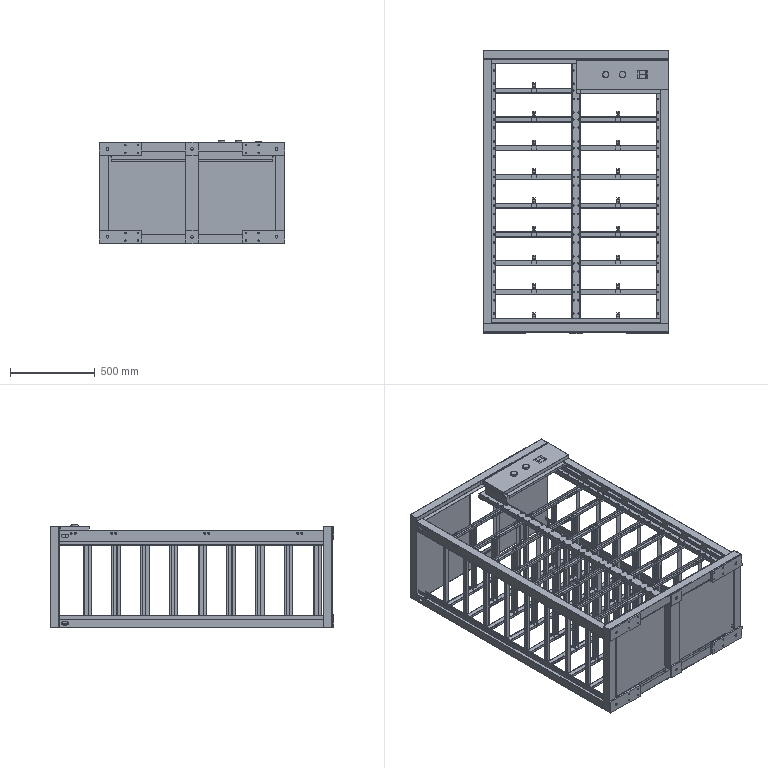Part | SolidWorks | features ReferencePattern 16, LocalLPattern 1 | 144 solids | 4696 faces | volume 11157281 mm3 | plane 3041 | cylinder 1599 | spline 56 | commonest cylinder face diameters 5.5 x320 0.2 x295 3.2 x281 4.5 x256 10.5 x162 9.5 x54